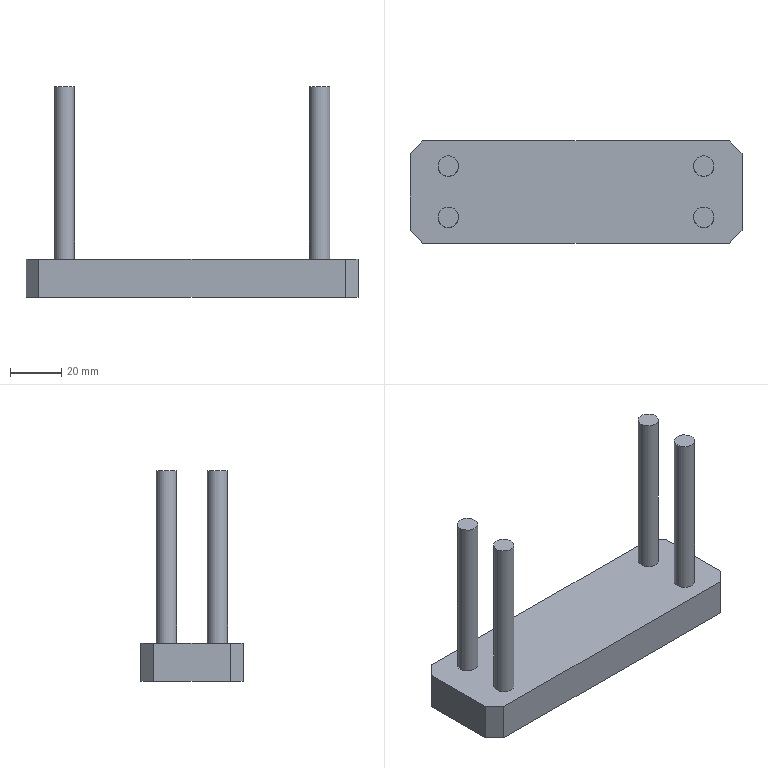Part | STEP file | Tube necking machine_id238_x_t | 1 solid | 18 faces | box 130 x 40 x 82.5 mm | volume 90822 mm3 | plane 14 | cylinder 4 | commonest cylinder face diameters 8 x4
STEP:
#1=CARTESIAN_POINT('',(0.,0.,0.));
#2=DIRECTION('',(0.,0.,1.));
#3=DIRECTION('',(1.,0.,0.));
#4=AXIS2_PLACEMENT_3D('',#1,#2,#3);
#5=CARTESIAN_POINT('',(-54.,60.,187.5));
#6=VERTEX_POINT('',#5);
#7=CARTESIAN_POINT('',(-46.,60.,187.5));
#8=VERTEX_POINT('',#7);
#9=CARTESIAN_POINT('',(-50.,60.,187.5));
#10=DIRECTION('',(0.,0.,-1.));
#11=DIRECTION('',(-1.,0.,0.));
#12=AXIS2_PLACEMENT_3D('',#9,#10,#11);
#13=CIRCLE('',#12,4.);
#14=CARTESIAN_POINT('',(-50.,60.,187.5));
#15=DIRECTION('',(0.,0.,-1.));
#16=DIRECTION('',(-1.,0.,0.));
#17=AXIS2_PLACEMENT_3D('',#14,#15,#16);
#18=PLANE('',#17);
#19=CARTESIAN_POINT('',(0.,0.));
#20=DIRECTION('',(1.,0.));
#21=AXIS2_PLACEMENT_2D('',#19,#20);
#22=CIRCLE('',#21,4.);
#23=(GEOMETRIC_REPRESENTATION_CONTEXT(2)PARAMETRIC_REPRESENTATION_CONTEXT()REPRESENTATION_CONTEXT('',''));
#24=DEFINITIONAL_REPRESENTATION('',(#22),#23);
#25=PCURVE('',#18,#24);
#26=CARTESIAN_POINT('',(-50.,60.,-489.65));
#27=DIRECTION('',(0.,0.,1.));
#28=DIRECTION('',(1.,0.,0.));
#29=AXIS2_PLACEMENT_3D('',#26,#27,#28);
#30=CYLINDRICAL_SURFACE('',#29,4.);
#31=CARTESIAN_POINT('',(3.142,677.15));
#32=DIRECTION('',(-1.,0.));
#33=VECTOR('',#32,1.);
#34=LINE('',#31,#33);
#35=(GEOMETRIC_REPRESENTATION_CONTEXT(2)PARAMETRIC_REPRESENTATION_CONTEXT()REPRESENTATION_CONTEXT('',''));
#36=DEFINITIONAL_REPRESENTATION('',(#34),#35);
#37=PCURVE('',#30,#36);
#38=SURFACE_CURVE('',#13,(#25,#37),.PCURVE_S1.);
#39=EDGE_CURVE('',#6,#8,#38,.T.);
#40=ORIENTED_EDGE('',*,*,#39,.F.);
#41=CARTESIAN_POINT('',(-50.,60.,187.5));
#42=DIRECTION('',(0.,0.,-1.));
#43=DIRECTION('',(-1.,0.,0.));
#44=AXIS2_PLACEMENT_3D('',#41,#42,#43);
#45=CIRCLE('',#44,4.);
#46=CARTESIAN_POINT('',(0.,0.));
#47=DIRECTION('',(1.,0.));
#48=AXIS2_PLACEMENT_2D('',#46,#47);
#49=CIRCLE('',#48,4.);
#50=(GEOMETRIC_REPRESENTATION_CONTEXT(2)PARAMETRIC_REPRESENTATION_CONTEXT()REPRESENTATION_CONTEXT('',''));
#51=DEFINITIONAL_REPRESENTATION('',(#49),#50);
#52=PCURVE('',#18,#51);
#53=CARTESIAN_POINT('',(9.425,677.15));
#54=DIRECTION('',(-1.,0.));
#55=VECTOR('',#54,1.);
#56=LINE('',#53,#55);
#57=(GEOMETRIC_REPRESENTATION_CONTEXT(2)PARAMETRIC_REPRESENTATION_CONTEXT()REPRESENTATION_CONTEXT('',''));
#58=DEFINITIONAL_REPRESENTATION('',(#56),#57);
#59=PCURVE('',#30,#58);
#60=SURFACE_CURVE('',#45,(#52,#59),.PCURVE_S1.);
#61=EDGE_CURVE('',#8,#6,#60,.T.);
#62=ORIENTED_EDGE('',*,*,#61,.F.);
#63=EDGE_LOOP('',(#40,#62));
#64=FACE_BOUND('',#63,.T.);
#65=ADVANCED_FACE('',(#64),#18,.F.);
#66=CARTESIAN_POINT('',(-46.,60.,120.));
#67=VERTEX_POINT('',#66);
#68=CARTESIAN_POINT('',(-50.,60.,120.));
#69=DIRECTION('',(0.,0.,1.));
#70=DIRECTION('',(1.,0.,0.));
#71=AXIS2_PLACEMENT_3D('',#68,#69,#70);
#72=CIRCLE('',#71,4.);
#73=CARTESIAN_POINT('',(0.,609.65));
#74=DIRECTION('',(1.,0.));
#75=VECTOR('',#74,1.);
#76=LINE('',#73,#75);
#77=(GEOMETRIC_REPRESENTATION_CONTEXT(2)PARAMETRIC_REPRESENTATION_CONTEXT()REPRESENTATION_CONTEXT('',''));
#78=DEFINITIONAL_REPRESENTATION('',(#76),#77);
#79=PCURVE('',#30,#78);
#80=CARTESIAN_POINT('',(0.,0.,120.));
#81=DIRECTION('',(0.,0.,1.));
#82=DIRECTION('',(1.,0.,0.));
#83=AXIS2_PLACEMENT_3D('',#80,#81,#82);
#84=PLANE('',#83);
#85=CARTESIAN_POINT('',(-50.,60.));
#86=DIRECTION('',(1.,0.));
#87=AXIS2_PLACEMENT_2D('',#85,#86);
#88=CIRCLE('',#87,4.);
#89=(GEOMETRIC_REPRESENTATION_CONTEXT(2)PARAMETRIC_REPRESENTATION_CONTEXT()REPRESENTATION_CONTEXT('',''));
#90=DEFINITIONAL_REPRESENTATION('',(#88),#89);
#91=PCURVE('',#84,#90);
#92=SURFACE_CURVE('',#72,(#79,#91),.PCURVE_S1.);
#93=EDGE_CURVE('',#67,#67,#92,.T.);
#94=ORIENTED_EDGE('',*,*,#93,.T.);
#95=CARTESIAN_POINT('',(-46.,60.,120.));
#96=CARTESIAN_POINT('',(-46.,60.,187.5));
#97=B_SPLINE_CURVE_WITH_KNOTS('',1,(#95,#96),.UNSPECIFIED.,.F.,.F.,(2,2),(609.65,677.15),.PIECEWISE_BEZIER_KNOTS.);
#98=CARTESIAN_POINT('',(6.283,0.));
#99=DIRECTION('',(0.,1.));
#100=VECTOR('',#99,1.);
#101=LINE('',#98,#100);
#102=(GEOMETRIC_REPRESENTATION_CONTEXT(2)PARAMETRIC_REPRESENTATION_CONTEXT()REPRESENTATION_CONTEXT('',''));
#103=DEFINITIONAL_REPRESENTATION('',(#101),#102);
#104=PCURVE('',#30,#103);
#105=CARTESIAN_POINT('',(0.,0.));
#106=DIRECTION('',(0.,1.));
#107=VECTOR('',#106,1.);
#108=LINE('',#105,#107);
#109=(GEOMETRIC_REPRESENTATION_CONTEXT(2)PARAMETRIC_REPRESENTATION_CONTEXT()REPRESENTATION_CONTEXT('',''));
#110=DEFINITIONAL_REPRESENTATION('',(#108),#109);
#111=PCURVE('',#30,#110);
#112=SEAM_CURVE('',#97,(#104,#111),.PCURVE_S1.);
#113=EDGE_CURVE('',#67,#8,#112,.T.);
#114=ORIENTED_EDGE('',*,*,#113,.T.);
#115=ORIENTED_EDGE('',*,*,#61,.T.);
#116=ORIENTED_EDGE('',*,*,#39,.T.);
#117=ORIENTED_EDGE('',*,*,#113,.F.);
#118=EDGE_LOOP('',(#94,#114,#115,#116,#117));
#119=FACE_BOUND('',#118,.T.);
#120=ADVANCED_FACE('',(#119),#30,.T.);
#121=CARTESIAN_POINT('',(-65.,65.,120.));
#122=VERTEX_POINT('',#121);
#123=CARTESIAN_POINT('',(-65.,35.,120.));
#124=VERTEX_POINT('',#123);
#125=CARTESIAN_POINT('',(-65.,70.,120.));
#126=DIRECTION('',(0.,-1.,0.));
#127=VECTOR('',#126,1.);
#128=LINE('',#125,#127);
#129=CARTESIAN_POINT('',(-65.,70.,120.));
#130=DIRECTION('',(1.,0.,0.));
#131=DIRECTION('',(0.,0.,-1.));
#132=AXIS2_PLACEMENT_3D('',#129,#130,#131);
#133=PLANE('',#132);
#134=CARTESIAN_POINT('',(0.,0.));
#135=DIRECTION('',(0.,-1.));
#136=VECTOR('',#135,1.);
#137=LINE('',#134,#136);
#138=(GEOMETRIC_REPRESENTATION_CONTEXT(2)PARAMETRIC_REPRESENTATION_CONTEXT()REPRESENTATION_CONTEXT('',''));
#139=DEFINITIONAL_REPRESENTATION('',(#137),#138);
#140=PCURVE('',#133,#139);
#141=CARTESIAN_POINT('',(-65.,70.));
#142=DIRECTION('',(0.,-1.));
#143=VECTOR('',#142,1.);
#144=LINE('',#141,#143);
#145=(GEOMETRIC_REPRESENTATION_CONTEXT(2)PARAMETRIC_REPRESENTATION_CONTEXT()REPRESENTATION_CONTEXT('',''));
#146=DEFINITIONAL_REPRESENTATION('',(#144),#145);
#147=PCURVE('',#84,#146);
#148=SURFACE_CURVE('',#128,(#140,#147),.PCURVE_S1.);
#149=EDGE_CURVE('',#122,#124,#148,.T.);
#150=ORIENTED_EDGE('',*,*,#149,.F.);
#151=CARTESIAN_POINT('',(-65.,65.,105.));
#152=VERTEX_POINT('',#151);
#153=CARTESIAN_POINT('',(-65.,65.,120.));
#154=DIRECTION('',(0.,0.,-1.));
#155=VECTOR('',#154,1.);
#156=LINE('',#153,#155);
#157=CARTESIAN_POINT('',(0.,-5.));
#158=DIRECTION('',(1.,0.));
#159=VECTOR('',#158,1.);
#160=LINE('',#157,#159);
#161=(GEOMETRIC_REPRESENTATION_CONTEXT(2)PARAMETRIC_REPRESENTATION_CONTEXT()REPRESENTATION_CONTEXT('',''));
#162=DEFINITIONAL_REPRESENTATION('',(#160),#161);
#163=PCURVE('',#133,#162);
#164=CARTESIAN_POINT('',(-65.,65.,120.));
#165=DIRECTION('',(0.7071,-0.7071,0.));
#166=DIRECTION('',(0.,0.,-1.));
#167=AXIS2_PLACEMENT_3D('',#164,#165,#166);
#168=PLANE('',#167);
#169=CARTESIAN_POINT('',(0.,0.));
#170=DIRECTION('',(1.,0.));
#171=VECTOR('',#170,1.);
#172=LINE('',#169,#171);
#173=(GEOMETRIC_REPRESENTATION_CONTEXT(2)PARAMETRIC_REPRESENTATION_CONTEXT()REPRESENTATION_CONTEXT('',''));
#174=DEFINITIONAL_REPRESENTATION('',(#172),#173);
#175=PCURVE('',#168,#174);
#176=SURFACE_CURVE('',#156,(#163,#175),.PCURVE_S1.);
#177=EDGE_CURVE('',#122,#152,#176,.T.);
#178=ORIENTED_EDGE('',*,*,#177,.T.);
#179=CARTESIAN_POINT('',(-65.,35.,105.));
#180=VERTEX_POINT('',#179);
#181=CARTESIAN_POINT('',(-65.,70.,105.));
#182=DIRECTION('',(0.,-1.,0.));
#183=VECTOR('',#182,1.);
#184=LINE('',#181,#183);
#185=CARTESIAN_POINT('',(15.,0.));
#186=DIRECTION('',(0.,-1.));
#187=VECTOR('',#186,1.);
#188=LINE('',#185,#187);
#189=(GEOMETRIC_REPRESENTATION_CONTEXT(2)PARAMETRIC_REPRESENTATION_CONTEXT()REPRESENTATION_CONTEXT('',''));
#190=DEFINITIONAL_REPRESENTATION('',(#188),#189);
#191=PCURVE('',#133,#190);
#192=CARTESIAN_POINT('',(0.,0.,105.));
#193=DIRECTION('',(0.,0.,1.));
#194=DIRECTION('',(1.,0.,0.));
#195=AXIS2_PLACEMENT_3D('',#192,#193,#194);
#196=PLANE('',#195);
#197=CARTESIAN_POINT('',(-65.,70.));
#198=DIRECTION('',(0.,-1.));
#199=VECTOR('',#198,1.);
#200=LINE('',#197,#199);
#201=(GEOMETRIC_REPRESENTATION_CONTEXT(2)PARAMETRIC_REPRESENTATION_CONTEXT()REPRESENTATION_CONTEXT('',''));
#202=DEFINITIONAL_REPRESENTATION('',(#200),#201);
#203=PCURVE('',#196,#202);
#204=SURFACE_CURVE('',#184,(#191,#203),.PCURVE_S1.);
#205=EDGE_CURVE('',#152,#180,#204,.T.);
#206=ORIENTED_EDGE('',*,*,#205,.T.);
#207=CARTESIAN_POINT('',(-65.,35.,120.));
#208=DIRECTION('',(0.,0.,1.));
#209=VECTOR('',#208,1.);
#210=LINE('',#207,#209);
#211=CARTESIAN_POINT('',(0.,-35.));
#212=DIRECTION('',(-1.,0.));
#213=VECTOR('',#212,1.);
#214=LINE('',#211,#213);
#215=(GEOMETRIC_REPRESENTATION_CONTEXT(2)PARAMETRIC_REPRESENTATION_CONTEXT()REPRESENTATION_CONTEXT('',''));
#216=DEFINITIONAL_REPRESENTATION('',(#214),#215);
#217=PCURVE('',#133,#216);
#218=CARTESIAN_POINT('',(-60.,30.,120.));
#219=DIRECTION('',(0.7071,0.7071,0.));
#220=DIRECTION('',(0.,0.,-1.));
#221=AXIS2_PLACEMENT_3D('',#218,#219,#220);
#222=PLANE('',#221);
#223=CARTESIAN_POINT('',(0.,7.071));
#224=DIRECTION('',(-1.,0.));
#225=VECTOR('',#224,1.);
#226=LINE('',#223,#225);
#227=(GEOMETRIC_REPRESENTATION_CONTEXT(2)PARAMETRIC_REPRESENTATION_CONTEXT()REPRESENTATION_CONTEXT('',''));
#228=DEFINITIONAL_REPRESENTATION('',(#226),#227);
#229=PCURVE('',#222,#228);
#230=SURFACE_CURVE('',#210,(#217,#229),.PCURVE_S1.);
#231=EDGE_CURVE('',#180,#124,#230,.T.);
#232=ORIENTED_EDGE('',*,*,#231,.T.);
#233=EDGE_LOOP('',(#150,#178,#206,#232));
#234=FACE_BOUND('',#233,.T.);
#235=ADVANCED_FACE('',(#234),#133,.F.);
#236=CARTESIAN_POINT('',(-60.,30.,120.));
#237=VERTEX_POINT('',#236);
#238=CARTESIAN_POINT('',(60.,30.,120.));
#239=VERTEX_POINT('',#238);
#240=CARTESIAN_POINT('',(-65.,30.,120.));
#241=DIRECTION('',(1.,0.,0.));
#242=VECTOR('',#241,1.);
#243=LINE('',#240,#242);
#244=CARTESIAN_POINT('',(-65.,30.,120.));
#245=DIRECTION('',(0.,1.,0.));
#246=DIRECTION('',(0.,0.,1.));
#247=AXIS2_PLACEMENT_3D('',#244,#245,#246);
#248=PLANE('',#247);
#249=CARTESIAN_POINT('',(0.,0.));
#250=DIRECTION('',(0.,1.));
#251=VECTOR('',#250,1.);
#252=LINE('',#249,#251);
#253=(GEOMETRIC_REPRESENTATION_CONTEXT(2)PARAMETRIC_REPRESENTATION_CONTEXT()REPRESENTATION_CONTEXT('',''));
#254=DEFINITIONAL_REPRESENTATION('',(#252),#253);
#255=PCURVE('',#248,#254);
#256=CARTESIAN_POINT('',(-65.,30.));
#257=DIRECTION('',(1.,0.));
#258=VECTOR('',#257,1.);
#259=LINE('',#256,#258);
#260=(GEOMETRIC_REPRESENTATION_CONTEXT(2)PARAMETRIC_REPRESENTATION_CONTEXT()REPRESENTATION_CONTEXT('',''));
#261=DEFINITIONAL_REPRESENTATION('',(#259),#260);
#262=PCURVE('',#84,#261);
#263=SURFACE_CURVE('',#243,(#255,#262),.PCURVE_S1.);
#264=EDGE_CURVE('',#237,#239,#263,.T.);
#265=ORIENTED_EDGE('',*,*,#264,.F.);
#266=CARTESIAN_POINT('',(-60.,30.,105.));
#267=VERTEX_POINT('',#266);
#268=CARTESIAN_POINT('',(-60.,30.,120.));
#269=DIRECTION('',(0.,0.,-1.));
#270=VECTOR('',#269,1.);
#271=LINE('',#268,#270);
#272=CARTESIAN_POINT('',(0.,5.));
#273=DIRECTION('',(-1.,0.));
#274=VECTOR('',#273,1.);
#275=LINE('',#272,#274);
#276=(GEOMETRIC_REPRESENTATION_CONTEXT(2)PARAMETRIC_REPRESENTATION_CONTEXT()REPRESENTATION_CONTEXT('',''));
#277=DEFINITIONAL_REPRESENTATION('',(#275),#276);
#278=PCURVE('',#248,#277);
#279=CARTESIAN_POINT('',(0.,0.));
#280=DIRECTION('',(1.,0.));
#281=VECTOR('',#280,1.);
#282=LINE('',#279,#281);
#283=(GEOMETRIC_REPRESENTATION_CONTEXT(2)PARAMETRIC_REPRESENTATION_CONTEXT()REPRESENTATION_CONTEXT('',''));
#284=DEFINITIONAL_REPRESENTATION('',(#282),#283);
#285=PCURVE('',#222,#284);
#286=SURFACE_CURVE('',#271,(#278,#285),.PCURVE_S1.);
#287=EDGE_CURVE('',#237,#267,#286,.T.);
#288=ORIENTED_EDGE('',*,*,#287,.T.);
#289=CARTESIAN_POINT('',(60.,30.,105.));
#290=VERTEX_POINT('',#289);
#291=CARTESIAN_POINT('',(-65.,30.,105.));
#292=DIRECTION('',(1.,0.,0.));
#293=VECTOR('',#292,1.);
#294=LINE('',#291,#293);
#295=CARTESIAN_POINT('',(-15.,0.));
#296=DIRECTION('',(0.,1.));
#297=VECTOR('',#296,1.);
#298=LINE('',#295,#297);
#299=(GEOMETRIC_REPRESENTATION_CONTEXT(2)PARAMETRIC_REPRESENTATION_CONTEXT()REPRESENTATION_CONTEXT('',''));
#300=DEFINITIONAL_REPRESENTATION('',(#298),#299);
#301=PCURVE('',#248,#300);
#302=CARTESIAN_POINT('',(-65.,30.));
#303=DIRECTION('',(1.,0.));
#304=VECTOR('',#303,1.);
#305=LINE('',#302,#304);
#306=(GEOMETRIC_REPRESENTATION_CONTEXT(2)PARAMETRIC_REPRESENTATION_CONTEXT()REPRESENTATION_CONTEXT('',''));
#307=DEFINITIONAL_REPRESENTATION('',(#305),#306);
#308=PCURVE('',#196,#307);
#309=SURFACE_CURVE('',#294,(#301,#308),.PCURVE_S1.);
#310=EDGE_CURVE('',#267,#290,#309,.T.);
#311=ORIENTED_EDGE('',*,*,#310,.T.);
#312=CARTESIAN_POINT('',(60.,30.,120.));
#313=DIRECTION('',(0.,0.,1.));
#314=VECTOR('',#313,1.);
#315=LINE('',#312,#314);
#316=CARTESIAN_POINT('',(0.,125.));
#317=DIRECTION('',(1.,0.));
#318=VECTOR('',#317,1.);
#319=LINE('',#316,#318);
#320=(GEOMETRIC_REPRESENTATION_CONTEXT(2)PARAMETRIC_REPRESENTATION_CONTEXT()REPRESENTATION_CONTEXT('',''));
#321=DEFINITIONAL_REPRESENTATION('',(#319),#320);
#322=PCURVE('',#248,#321);
#323=CARTESIAN_POINT('',(65.,35.,120.));
#324=DIRECTION('',(-0.7071,0.7071,0.));
#325=DIRECTION('',(0.,0.,-1.));
#326=AXIS2_PLACEMENT_3D('',#323,#324,#325);
#327=PLANE('',#326);
#328=CARTESIAN_POINT('',(0.,7.071));
#329=DIRECTION('',(-1.,0.));
#330=VECTOR('',#329,1.);
#331=LINE('',#328,#330);
#332=(GEOMETRIC_REPRESENTATION_CONTEXT(2)PARAMETRIC_REPRESENTATION_CONTEXT()REPRESENTATION_CONTEXT('',''));
#333=DEFINITIONAL_REPRESENTATION('',(#331),#332);
#334=PCURVE('',#327,#333);
#335=SURFACE_CURVE('',#315,(#322,#334),.PCURVE_S1.);
#336=EDGE_CURVE('',#290,#239,#335,.T.);
#337=ORIENTED_EDGE('',*,*,#336,.T.);
#338=EDGE_LOOP('',(#265,#288,#311,#337));
#339=FACE_BOUND('',#338,.T.);
#340=ADVANCED_FACE('',(#339),#248,.F.);
#341=CARTESIAN_POINT('',(65.,35.,105.));
#342=VERTEX_POINT('',#341);
#343=CARTESIAN_POINT('',(65.,65.,105.));
#344=VERTEX_POINT('',#343);
#345=CARTESIAN_POINT('',(65.,30.,105.));
#346=DIRECTION('',(0.,1.,0.));
#347=VECTOR('',#346,1.);
#348=LINE('',#345,#347);
#349=CARTESIAN_POINT('',(65.,30.,120.));
#350=DIRECTION('',(-1.,0.,0.));
#351=DIRECTION('',(0.,0.,1.));
#352=AXIS2_PLACEMENT_3D('',#349,#350,#351);
#353=PLANE('',#352);
#354=CARTESIAN_POINT('',(-15.,0.));
#355=DIRECTION('',(0.,1.));
#356=VECTOR('',#355,1.);
#357=LINE('',#354,#356);
#358=(GEOMETRIC_REPRESENTATION_CONTEXT(2)PARAMETRIC_REPRESENTATION_CONTEXT()REPRESENTATION_CONTEXT('',''));
#359=DEFINITIONAL_REPRESENTATION('',(#357),#358);
#360=PCURVE('',#353,#359);
#361=CARTESIAN_POINT('',(65.,30.));
#362=DIRECTION('',(0.,1.));
#363=VECTOR('',#362,1.);
#364=LINE('',#361,#363);
#365=(GEOMETRIC_REPRESENTATION_CONTEXT(2)PARAMETRIC_REPRESENTATION_CONTEXT()REPRESENTATION_CONTEXT('',''));
#366=DEFINITIONAL_REPRESENTATION('',(#364),#365);
#367=PCURVE('',#196,#366);
#368=SURFACE_CURVE('',#348,(#360,#367),.PCURVE_S1.);
#369=EDGE_CURVE('',#342,#344,#368,.T.);
#370=ORIENTED_EDGE('',*,*,#369,.T.);
#371=CARTESIAN_POINT('',(65.,65.,120.));
#372=VERTEX_POINT('',#371);
#373=CARTESIAN_POINT('',(65.,65.,120.));
#374=DIRECTION('',(0.,0.,1.));
#375=VECTOR('',#374,1.);
#376=LINE('',#373,#375);
#377=CARTESIAN_POINT('',(0.,35.));
#378=DIRECTION('',(1.,0.));
#379=VECTOR('',#378,1.);
#380=LINE('',#377,#379);
#381=(GEOMETRIC_REPRESENTATION_CONTEXT(2)PARAMETRIC_REPRESENTATION_CONTEXT()REPRESENTATION_CONTEXT('',''));
#382=DEFINITIONAL_REPRESENTATION('',(#380),#381);
#383=PCURVE('',#353,#382);
#384=CARTESIAN_POINT('',(60.,70.,120.));
#385=DIRECTION('',(-0.7071,-0.7071,0.));
#386=DIRECTION('',(0.,0.,-1.));
#387=AXIS2_PLACEMENT_3D('',#384,#385,#386);
#388=PLANE('',#387);
#389=CARTESIAN_POINT('',(0.,7.071));
#390=DIRECTION('',(-1.,0.));
#391=VECTOR('',#390,1.);
#392=LINE('',#389,#391);
#393=(GEOMETRIC_REPRESENTATION_CONTEXT(2)PARAMETRIC_REPRESENTATION_CONTEXT()REPRESENTATION_CONTEXT('',''));
#394=DEFINITIONAL_REPRESENTATION('',(#392),#393);
#395=PCURVE('',#388,#394);
#396=SURFACE_CURVE('',#376,(#383,#395),.PCURVE_S1.);
#397=EDGE_CURVE('',#344,#372,#396,.T.);
#398=ORIENTED_EDGE('',*,*,#397,.T.);
#399=CARTESIAN_POINT('',(65.,35.,120.));
#400=VERTEX_POINT('',#399);
#401=CARTESIAN_POINT('',(65.,30.,120.));
#402=DIRECTION('',(0.,1.,0.));
#403=VECTOR('',#402,1.);
#404=LINE('',#401,#403);
#405=CARTESIAN_POINT('',(0.,0.));
#406=DIRECTION('',(0.,1.));
#407=VECTOR('',#406,1.);
#408=LINE('',#405,#407);
#409=(GEOMETRIC_REPRESENTATION_CONTEXT(2)PARAMETRIC_REPRESENTATION_CONTEXT()REPRESENTATION_CONTEXT('',''));
#410=DEFINITIONAL_REPRESENTATION('',(#408),#409);
#411=PCURVE('',#353,#410);
#412=CARTESIAN_POINT('',(65.,30.));
#413=DIRECTION('',(0.,1.));
#414=VECTOR('',#413,1.);
#415=LINE('',#412,#414);
#416=(GEOMETRIC_REPRESENTATION_CONTEXT(2)PARAMETRIC_REPRESENTATION_CONTEXT()REPRESENTATION_CONTEXT('',''));
#417=DEFINITIONAL_REPRESENTATION('',(#415),#416);
#418=PCURVE('',#84,#417);
#419=SURFACE_CURVE('',#404,(#411,#418),.PCURVE_S1.);
#420=EDGE_CURVE('',#400,#372,#419,.T.);
#421=ORIENTED_EDGE('',*,*,#420,.F.);
#422=CARTESIAN_POINT('',(65.,35.,120.));
#423=DIRECTION('',(0.,0.,-1.));
#424=VECTOR('',#423,1.);
#425=LINE('',#422,#424);
#426=CARTESIAN_POINT('',(0.,5.));
#427=DIRECTION('',(-1.,0.));
#428=VECTOR('',#427,1.);
#429=LINE('',#426,#428);
#430=(GEOMETRIC_REPRESENTATION_CONTEXT(2)PARAMETRIC_REPRESENTATION_CONTEXT()REPRESENTATION_CONTEXT('',''));
#431=DEFINITIONAL_REPRESENTATION('',(#429),#430);
#432=PCURVE('',#353,#431);
#433=CARTESIAN_POINT('',(0.,0.));
#434=DIRECTION('',(1.,0.));
#435=VECTOR('',#434,1.);
#436=LINE('',#433,#435);
#437=(GEOMETRIC_REPRESENTATION_CONTEXT(2)PARAMETRIC_REPRESENTATION_CONTEXT()REPRESENTATION_CONTEXT('',''));
#438=DEFINITIONAL_REPRESENTATION('',(#436),#437);
#439=PCURVE('',#327,#438);
#440=SURFACE_CURVE('',#425,(#432,#439),.PCURVE_S1.);
#441=EDGE_CURVE('',#400,#342,#440,.T.);
#442=ORIENTED_EDGE('',*,*,#441,.T.);
#443=EDGE_LOOP('',(#370,#398,#421,#442));
#444=FACE_BOUND('',#443,.T.);
#445=ADVANCED_FACE('',(#444),#353,.F.);
#446=CARTESIAN_POINT('',(60.,70.,105.));
#447=VERTEX_POINT('',#446);
#448=CARTESIAN_POINT('',(-60.,70.,105.));
#449=VERTEX_POINT('',#448);
#450=CARTESIAN_POINT('',(65.,70.,105.));
#451=DIRECTION('',(-1.,0.,0.));
#452=VECTOR('',#451,1.);
#453=LINE('',#450,#452);
#454=CARTESIAN_POINT('',(65.,70.,120.));
#455=DIRECTION('',(0.,-1.,0.));
#456=DIRECTION('',(0.,0.,-1.));
#457=AXIS2_PLACEMENT_3D('',#454,#455,#456);
#458=PLANE('',#457);
#459=CARTESIAN_POINT('',(15.,0.));
#460=DIRECTION('',(0.,-1.));
#461=VECTOR('',#460,1.);
#462=LINE('',#459,#461);
#463=(GEOMETRIC_REPRESENTATION_CONTEXT(2)PARAMETRIC_REPRESENTATION_CONTEXT()REPRESENTATION_CONTEXT('',''));
#464=DEFINITIONAL_REPRESENTATION('',(#462),#463);
#465=PCURVE('',#458,#464);
#466=CARTESIAN_POINT('',(65.,70.));
#467=DIRECTION('',(-1.,0.));
#468=VECTOR('',#467,1.);
#469=LINE('',#466,#468);
#470=(GEOMETRIC_REPRESENTATION_CONTEXT(2)PARAMETRIC_REPRESENTATION_CONTEXT()REPRESENTATION_CONTEXT('',''));
#471=DEFINITIONAL_REPRESENTATION('',(#469),#470);
#472=PCURVE('',#196,#471);
#473=SURFACE_CURVE('',#453,(#465,#472),.PCURVE_S1.);
#474=EDGE_CURVE('',#447,#449,#473,.T.);
#475=ORIENTED_EDGE('',*,*,#474,.T.);
#476=CARTESIAN_POINT('',(-60.,70.,120.));
#477=VERTEX_POINT('',#476);
#478=CARTESIAN_POINT('',(-60.,70.,120.));
#479=DIRECTION('',(0.,0.,1.));
#480=VECTOR('',#479,1.);
#481=LINE('',#478,#480);
#482=CARTESIAN_POINT('',(0.,-125.));
#483=DIRECTION('',(-1.,0.));
#484=VECTOR('',#483,1.);
#485=LINE('',#482,#484);
#486=(GEOMETRIC_REPRESENTATION_CONTEXT(2)PARAMETRIC_REPRESENTATION_CONTEXT()REPRESENTATION_CONTEXT('',''));
#487=DEFINITIONAL_REPRESENTATION('',(#485),#486);
#488=PCURVE('',#458,#487);
#489=CARTESIAN_POINT('',(0.,7.071));
#490=DIRECTION('',(-1.,0.));
#491=VECTOR('',#490,1.);
#492=LINE('',#489,#491);
#493=(GEOMETRIC_REPRESENTATION_CONTEXT(2)PARAMETRIC_REPRESENTATION_CONTEXT()REPRESENTATION_CONTEXT('',''));
#494=DEFINITIONAL_REPRESENTATION('',(#492),#493);
#495=PCURVE('',#168,#494);
#496=SURFACE_CURVE('',#481,(#488,#495),.PCURVE_S1.);
#497=EDGE_CURVE('',#449,#477,#496,.T.);
#498=ORIENTED_EDGE('',*,*,#497,.T.);
#499=CARTESIAN_POINT('',(60.,70.,120.));
#500=VERTEX_POINT('',#499);
#501=CARTESIAN_POINT('',(65.,70.,120.));
#502=DIRECTION('',(-1.,0.,0.));
#503=VECTOR('',#502,1.);
#504=LINE('',#501,#503);
#505=CARTESIAN_POINT('',(0.,0.));
#506=DIRECTION('',(0.,-1.));
#507=VECTOR('',#506,1.);
#508=LINE('',#505,#507);
#509=(GEOMETRIC_REPRESENTATION_CONTEXT(2)PARAMETRIC_REPRESENTATION_CONTEXT()REPRESENTATION_CONTEXT('',''));
#510=DEFINITIONAL_REPRESENTATION('',(#508),#509);
#511=PCURVE('',#458,#510);
#512=CARTESIAN_POINT('',(65.,70.));
#513=DIRECTION('',(-1.,0.));
#514=VECTOR('',#513,1.);
#515=LINE('',#512,#514);
#516=(GEOMETRIC_REPRESENTATION_CONTEXT(2)PARAMETRIC_REPRESENTATION_CONTEXT()REPRESENTATION_CONTEXT('',''));
#517=DEFINITIONAL_REPRESENTATION('',(#515),#516);
#518=PCURVE('',#84,#517);
#519=SURFACE_CURVE('',#504,(#511,#518),.PCURVE_S1.);
#520=EDGE_CURVE('',#500,#477,#519,.T.);
#521=ORIENTED_EDGE('',*,*,#520,.F.);
#522=CARTESIAN_POINT('',(60.,70.,120.));
#523=DIRECTION('',(0.,0.,-1.));
#524=VECTOR('',#523,1.);
#525=LINE('',#522,#524);
#526=CARTESIAN_POINT('',(0.,-5.));
#527=DIRECTION('',(1.,0.));
#528=VECTOR('',#527,1.);
#529=LINE('',#526,#528);
#530=(GEOMETRIC_REPRESENTATION_CONTEXT(2)PARAMETRIC_REPRESENTATION_CONTEXT()REPRESENTATION_CONTEXT('',''));
#531=DEFINITIONAL_REPRESENTATION('',(#529),#530);
#532=PCURVE('',#458,#531);
#533=CARTESIAN_POINT('',(0.,0.));
#534=DIRECTION('',(1.,0.));
#535=VECTOR('',#534,1.);
#536=LINE('',#533,#535);
#537=(GEOMETRIC_REPRESENTATION_CONTEXT(2)PARAMETRIC_REPRESENTATION_CONTEXT()REPRESENTATION_CONTEXT('',''));
#538=DEFINITIONAL_REPRESENTATION('',(#536),#537);
#539=PCURVE('',#388,#538);
#540=SURFACE_CURVE('',#525,(#532,#539),.PCURVE_S1.);
#541=EDGE_CURVE('',#500,#447,#540,.T.);
#542=ORIENTED_EDGE('',*,*,#541,.T.);
#543=EDGE_LOOP('',(#475,#498,#521,#542));
#544=FACE_BOUND('',#543,.T.);
#545=ADVANCED_FACE('',(#544),#458,.F.);
#546=ORIENTED_EDGE('',*,*,#93,.F.);
#547=EDGE_LOOP('',(#546));
#548=FACE_BOUND('',#547,.T.);
#549=CARTESIAN_POINT('',(54.,60.,120.));
#550=VERTEX_POINT('',#549);
#551=CARTESIAN_POINT('',(50.,60.,120.));
#552=DIRECTION('',(0.,0.,1.));
#553=DIRECTION('',(1.,0.,0.));
#554=AXIS2_PLACEMENT_3D('',#551,#552,#553);
#555=CIRCLE('',#554,4.);
#556=CARTESIAN_POINT('',(50.,60.));
#557=DIRECTION('',(1.,0.));
#558=AXIS2_PLACEMENT_2D('',#556,#557);
#559=CIRCLE('',#558,4.);
#560=(GEOMETRIC_REPRESENTATION_CONTEXT(2)PARAMETRIC_REPRESENTATION_CONTEXT()REPRESENTATION_CONTEXT('',''));
#561=DEFINITIONAL_REPRESENTATION('',(#559),#560);
#562=PCURVE('',#84,#561);
#563=CARTESIAN_POINT('',(50.,60.,-489.65));
#564=DIRECTION('',(0.,0.,1.));
#565=DIRECTION('',(1.,0.,0.));
#566=AXIS2_PLACEMENT_3D('',#563,#564,#565);
#567=CYLINDRICAL_SURFACE('',#566,4.);
#568=CARTESIAN_POINT('',(0.,609.65));
#569=DIRECTION('',(1.,0.));
#570=VECTOR('',#569,1.);
#571=LINE('',#568,#570);
#572=(GEOMETRIC_REPRESENTATION_CONTEXT(2)PARAMETRIC_REPRESENTATION_CONTEXT()REPRESENTATION_CONTEXT('',''));
#573=DEFINITIONAL_REPRESENTATION('',(#571),#572);
#574=PCURVE('',#567,#573);
#575=SURFACE_CURVE('',#555,(#562,#574),.PCURVE_S1.);
#576=EDGE_CURVE('',#550,#550,#575,.T.);
#577=ORIENTED_EDGE('',*,*,#576,.F.);
#578=EDGE_LOOP('',(#577));
#579=FACE_BOUND('',#578,.T.);
#580=CARTESIAN_POINT('',(54.,40.,120.));
#581=VERTEX_POINT('',#580);
#582=CARTESIAN_POINT('',(50.,40.,120.));
#583=DIRECTION('',(0.,0.,-1.));
#584=DIRECTION('',(1.,0.,0.));
#585=AXIS2_PLACEMENT_3D('',#582,#583,#584);
#586=CIRCLE('',#585,4.);
#587=CARTESIAN_POINT('',(54.,40.));
#588=CARTESIAN_POINT('',(54.,33.072));
#589=CARTESIAN_POINT('',(48.,36.536));
#590=CARTESIAN_POINT('',(42.,40.));
#591=CARTESIAN_POINT('',(48.,43.464));
#592=CARTESIAN_POINT('',(54.,46.928));
#593=CARTESIAN_POINT('',(54.,40.));
#594=(BOUNDED_CURVE()B_SPLINE_CURVE(2,(#587,#588,#589,#590,#591,#592,#593),.UNSPECIFIED.,.T.,.F.)B_SPLINE_CURVE_WITH_KNOTS((1,2,2,2,2,1),(-2.094,0.,2.094,4.189,6.283,8.378),.UNSPECIFIED.)CURVE()GEOMETRIC_REPRESENTATION_ITEM()RATIONAL_B_SPLINE_CURVE((1.,0.5,1.,0.5,1.,0.5,1.))REPRESENTATION_ITEM(''));
#595=(GEOMETRIC_REPRESENTATION_CONTEXT(2)PARAMETRIC_REPRESENTATION_CONTEXT()REPRESENTATION_CONTEXT('',''));
#596=DEFINITIONAL_REPRESENTATION('',(#594),#595);
#597=PCURVE('',#84,#596);
#598=CARTESIAN_POINT('',(50.,40.,-489.65));
#599=DIRECTION('',(0.,0.,1.));
#600=DIRECTION('',(1.,0.,0.));
#601=AXIS2_PLACEMENT_3D('',#598,#599,#600);
#602=CYLINDRICAL_SURFACE('',#601,4.);
#603=CARTESIAN_POINT('',(6.283,609.65));
#604=DIRECTION('',(-1.,0.));
#605=VECTOR('',#604,1.);
#606=LINE('',#603,#605);
#607=(GEOMETRIC_REPRESENTATION_CONTEXT(2)PARAMETRIC_REPRESENTATION_CONTEXT()REPRESENTATION_CONTEXT('',''));
#608=DEFINITIONAL_REPRESENTATION('',(#606),#607);
#609=PCURVE('',#602,#608);
#610=SURFACE_CURVE('',#586,(#597,#609),.PCURVE_S1.);
#611=EDGE_CURVE('',#581,#581,#610,.T.);
#612=ORIENTED_EDGE('',*,*,#611,.T.);
#613=EDGE_LOOP('',(#612));
#614=FACE_BOUND('',#613,.T.);
#615=CARTESIAN_POINT('',(-46.,40.,120.));
#616=VERTEX_POINT('',#615);
#617=CARTESIAN_POINT('',(-50.,40.,120.));
#618=DIRECTION('',(0.,0.,1.));
#619=DIRECTION('',(1.,0.,0.));
#620=AXIS2_PLACEMENT_3D('',#617,#618,#619);
#621=CIRCLE('',#620,4.);
#622=CARTESIAN_POINT('',(-50.,40.));
#623=DIRECTION('',(1.,0.));
#624=AXIS2_PLACEMENT_2D('',#622,#623);
#625=CIRCLE('',#624,4.);
#626=(GEOMETRIC_REPRESENTATION_CONTEXT(2)PARAMETRIC_REPRESENTATION_CONTEXT()REPRESENTATION_CONTEXT('',''));
#627=DEFINITIONAL_REPRESENTATION('',(#625),#626);
#628=PCURVE('',#84,#627);
#629=CARTESIAN_POINT('',(-50.,40.,-489.65));
#630=DIRECTION('',(0.,0.,1.));
#631=DIRECTION('',(1.,0.,0.));
#632=AXIS2_PLACEMENT_3D('',#629,#630,#631);
#633=CYLINDRICAL_SURFACE('',#632,4.);
#634=CARTESIAN_POINT('',(0.,609.65));
#635=DIRECTION('',(1.,0.));
#636=VECTOR('',#635,1.);
#637=LINE('',#634,#636);
#638=(GEOMETRIC_REPRESENTATION_CONTEXT(2)PARAMETRIC_REPRESENTATION_CONTEXT()REPRESENTATION_CONTEXT('',''));
#639=DEFINITIONAL_REPRESENTATION('',(#637),#638);
#640=PCURVE('',#633,#639);
#641=SURFACE_CURVE('',#621,(#628,#640),.PCURVE_S1.);
#642=EDGE_CURVE('',#616,#616,#641,.T.);
#643=ORIENTED_EDGE('',*,*,#642,.F.);
#644=EDGE_LOOP('',(#643));
#645=FACE_BOUND('',#644,.T.);
#646=ORIENTED_EDGE('',*,*,#520,.T.);
#647=CARTESIAN_POINT('',(-65.,65.,120.));
#648=DIRECTION('',(-0.7071,-0.7071,0.));
#649=VECTOR('',#648,1.);
#650=LINE('',#647,#649);
#651=CARTESIAN_POINT('',(-65.,65.));
#652=DIRECTION('',(-0.7071,-0.7071));
#653=VECTOR('',#652,1.);
#654=LINE('',#651,#653);
#655=(GEOMETRIC_REPRESENTATION_CONTEXT(2)PARAMETRIC_REPRESENTATION_CONTEXT()REPRESENTATION_CONTEXT('',''));
#656=DEFINITIONAL_REPRESENTATION('',(#654),#655);
#657=PCURVE('',#84,#656);
#658=CARTESIAN_POINT('',(0.,0.));
#659=DIRECTION('',(0.,-1.));
#660=VECTOR('',#659,1.);
#661=LINE('',#658,#660);
#662=(GEOMETRIC_REPRESENTATION_CONTEXT(2)PARAMETRIC_REPRESENTATION_CONTEXT()REPRESENTATION_CONTEXT('',''));
#663=DEFINITIONAL_REPRESENTATION('',(#661),#662);
#664=PCURVE('',#168,#663);
#665=SURFACE_CURVE('',#650,(#657,#664),.PCURVE_S1.);
#666=EDGE_CURVE('',#477,#122,#665,.T.);
#667=ORIENTED_EDGE('',*,*,#666,.T.);
#668=ORIENTED_EDGE('',*,*,#149,.T.);
#669=CARTESIAN_POINT('',(-15.,-15.,120.));
#670=DIRECTION('',(0.7071,-0.7071,0.));
#671=VECTOR('',#670,1.);
#672=LINE('',#669,#671);
#673=CARTESIAN_POINT('',(-15.,-15.));
#674=DIRECTION('',(0.7071,-0.7071));
#675=VECTOR('',#674,1.);
#676=LINE('',#673,#675);
#677=(GEOMETRIC_REPRESENTATION_CONTEXT(2)PARAMETRIC_REPRESENTATION_CONTEXT()REPRESENTATION_CONTEXT('',''));
#678=DEFINITIONAL_REPRESENTATION('',(#676),#677);
#679=PCURVE('',#84,#678);
#680=CARTESIAN_POINT('',(0.,-63.64));
#681=DIRECTION('',(0.,-1.));
#682=VECTOR('',#681,1.);
#683=LINE('',#680,#682);
#684=(GEOMETRIC_REPRESENTATION_CONTEXT(2)PARAMETRIC_REPRESENTATION_CONTEXT()REPRESENTATION_CONTEXT('',''));
#685=DEFINITIONAL_REPRESENTATION('',(#683),#684);
#686=PCURVE('',#222,#685);
#687=SURFACE_CURVE('',#672,(#679,#686),.PCURVE_S1.);
#688=EDGE_CURVE('',#124,#237,#687,.T.);
#689=ORIENTED_EDGE('',*,*,#688,.T.);
#690=ORIENTED_EDGE('',*,*,#264,.T.);
#691=CARTESIAN_POINT('',(15.,-15.,120.));
#692=DIRECTION('',(0.7071,0.7071,0.));
#693=VECTOR('',#692,1.);
#694=LINE('',#691,#693);
#695=CARTESIAN_POINT('',(15.,-15.));
#696=DIRECTION('',(0.7071,0.7071));
#697=VECTOR('',#696,1.);
#698=LINE('',#695,#697);
#699=(GEOMETRIC_REPRESENTATION_CONTEXT(2)PARAMETRIC_REPRESENTATION_CONTEXT()REPRESENTATION_CONTEXT('',''));
#700=DEFINITIONAL_REPRESENTATION('',(#698),#699);
#701=PCURVE('',#84,#700);
#702=CARTESIAN_POINT('',(0.,70.711));
#703=DIRECTION('',(0.,-1.));
#704=VECTOR('',#703,1.);
#705=LINE('',#702,#704);
#706=(GEOMETRIC_REPRESENTATION_CONTEXT(2)PARAMETRIC_REPRESENTATION_CONTEXT()REPRESENTATION_CONTEXT('',''));
#707=DEFINITIONAL_REPRESENTATION('',(#705),#706);
#708=PCURVE('',#327,#707);
#709=SURFACE_CURVE('',#694,(#701,#708),.PCURVE_S1.);
#710=EDGE_CURVE('',#239,#400,#709,.T.);
#711=ORIENTED_EDGE('',*,*,#710,.T.);
#712=ORIENTED_EDGE('',*,*,#420,.T.);
#713=CARTESIAN_POINT('',(65.,65.,120.));
#714=DIRECTION('',(-0.7071,0.7071,0.));
#715=VECTOR('',#714,1.);
#716=LINE('',#713,#715);
#717=CARTESIAN_POINT('',(65.,65.));
#718=DIRECTION('',(-0.7071,0.7071));
#719=VECTOR('',#718,1.);
#720=LINE('',#717,#719);
#721=(GEOMETRIC_REPRESENTATION_CONTEXT(2)PARAMETRIC_REPRESENTATION_CONTEXT()REPRESENTATION_CONTEXT('',''));
#722=DEFINITIONAL_REPRESENTATION('',(#720),#721);
#723=PCURVE('',#84,#722);
#724=CARTESIAN_POINT('',(0.,7.071));
#725=DIRECTION('',(0.,-1.));
#726=VECTOR('',#725,1.);
#727=LINE('',#724,#726);
#728=(GEOMETRIC_REPRESENTATION_CONTEXT(2)PARAMETRIC_REPRESENTATION_CONTEXT()REPRESENTATION_CONTEXT('',''));
#729=DEFINITIONAL_REPRESENTATION('',(#727),#728);
#730=PCURVE('',#388,#729);
#731=SURFACE_CURVE('',#716,(#723,#730),.PCURVE_S1.);
#732=EDGE_CURVE('',#372,#500,#731,.T.);
#733=ORIENTED_EDGE('',*,*,#732,.T.);
#734=EDGE_LOOP('',(#646,#667,#668,#689,#690,#711,#712,#733));
#735=FACE_BOUND('',#734,.T.);
#736=ADVANCED_FACE('',(#548,#579,#614,#645,#735),#84,.T.);
#737=ORIENTED_EDGE('',*,*,#205,.F.);
#738=CARTESIAN_POINT('',(-65.,65.,105.));
#739=DIRECTION('',(0.7071,0.7071,0.));
#740=VECTOR('',#739,1.);
#741=LINE('',#738,#740);
#742=CARTESIAN_POINT('',(-65.,65.));
#743=DIRECTION('',(0.7071,0.7071));
#744=VECTOR('',#743,1.);
#745=LINE('',#742,#744);
#746=(GEOMETRIC_REPRESENTATION_CONTEXT(2)PARAMETRIC_REPRESENTATION_CONTEXT()REPRESENTATION_CONTEXT('',''));
#747=DEFINITIONAL_REPRESENTATION('',(#745),#746);
#748=PCURVE('',#196,#747);
#749=CARTESIAN_POINT('',(15.,0.));
#750=DIRECTION('',(0.,1.));
#751=VECTOR('',#750,1.);
#752=LINE('',#749,#751);
#753=(GEOMETRIC_REPRESENTATION_CONTEXT(2)PARAMETRIC_REPRESENTATION_CONTEXT()REPRESENTATION_CONTEXT('',''));
#754=DEFINITIONAL_REPRESENTATION('',(#752),#753);
#755=PCURVE('',#168,#754);
#756=SURFACE_CURVE('',#741,(#748,#755),.PCURVE_S1.);
#757=EDGE_CURVE('',#152,#449,#756,.T.);
#758=ORIENTED_EDGE('',*,*,#757,.T.);
#759=ORIENTED_EDGE('',*,*,#474,.F.);
#760=CARTESIAN_POINT('',(60.,70.,105.));
#761=DIRECTION('',(0.7071,-0.7071,0.));
#762=VECTOR('',#761,1.);
#763=LINE('',#760,#762);
#764=CARTESIAN_POINT('',(60.,70.));
#765=DIRECTION('',(0.7071,-0.7071));
#766=VECTOR('',#765,1.);
#767=LINE('',#764,#766);
#768=(GEOMETRIC_REPRESENTATION_CONTEXT(2)PARAMETRIC_REPRESENTATION_CONTEXT()REPRESENTATION_CONTEXT('',''));
#769=DEFINITIONAL_REPRESENTATION('',(#767),#768);
#770=PCURVE('',#196,#769);
#771=CARTESIAN_POINT('',(15.,0.));
#772=DIRECTION('',(0.,1.));
#773=VECTOR('',#772,1.);
#774=LINE('',#771,#773);
#775=(GEOMETRIC_REPRESENTATION_CONTEXT(2)PARAMETRIC_REPRESENTATION_CONTEXT()REPRESENTATION_CONTEXT('',''));
#776=DEFINITIONAL_REPRESENTATION('',(#774),#775);
#777=PCURVE('',#388,#776);
#778=SURFACE_CURVE('',#763,(#770,#777),.PCURVE_S1.);
#779=EDGE_CURVE('',#447,#344,#778,.T.);
#780=ORIENTED_EDGE('',*,*,#779,.T.);
#781=ORIENTED_EDGE('',*,*,#369,.F.);
#782=CARTESIAN_POINT('',(65.,35.,105.));
#783=DIRECTION('',(-0.7071,-0.7071,0.));
#784=VECTOR('',#783,1.);
#785=LINE('',#782,#784);
#786=CARTESIAN_POINT('',(65.,35.));
#787=DIRECTION('',(-0.7071,-0.7071));
#788=VECTOR('',#787,1.);
#789=LINE('',#786,#788);
#790=(GEOMETRIC_REPRESENTATION_CONTEXT(2)PARAMETRIC_REPRESENTATION_CONTEXT()REPRESENTATION_CONTEXT('',''));
#791=DEFINITIONAL_REPRESENTATION('',(#789),#790);
#792=PCURVE('',#196,#791);
#793=CARTESIAN_POINT('',(15.,0.));
#794=DIRECTION('',(0.,1.));
#795=VECTOR('',#794,1.);
#796=LINE('',#793,#795);
#797=(GEOMETRIC_REPRESENTATION_CONTEXT(2)PARAMETRIC_REPRESENTATION_CONTEXT()REPRESENTATION_CONTEXT('',''));
#798=DEFINITIONAL_REPRESENTATION('',(#796),#797);
#799=PCURVE('',#327,#798);
#800=SURFACE_CURVE('',#785,(#792,#799),.PCURVE_S1.);
#801=EDGE_CURVE('',#342,#290,#800,.T.);
#802=ORIENTED_EDGE('',*,*,#801,.T.);
#803=ORIENTED_EDGE('',*,*,#310,.F.);
#804=CARTESIAN_POINT('',(-60.,30.,105.));
#805=DIRECTION('',(-0.7071,0.7071,0.));
#806=VECTOR('',#805,1.);
#807=LINE('',#804,#806);
#808=CARTESIAN_POINT('',(-60.,30.));
#809=DIRECTION('',(-0.7071,0.7071));
#810=VECTOR('',#809,1.);
#811=LINE('',#808,#810);
#812=(GEOMETRIC_REPRESENTATION_CONTEXT(2)PARAMETRIC_REPRESENTATION_CONTEXT()REPRESENTATION_CONTEXT('',''));
#813=DEFINITIONAL_REPRESENTATION('',(#811),#812);
#814=PCURVE('',#196,#813);
#815=CARTESIAN_POINT('',(15.,0.));
#816=DIRECTION('',(0.,1.));
#817=VECTOR('',#816,1.);
#818=LINE('',#815,#817);
#819=(GEOMETRIC_REPRESENTATION_CONTEXT(2)PARAMETRIC_REPRESENTATION_CONTEXT()REPRESENTATION_CONTEXT('',''));
#820=DEFINITIONAL_REPRESENTATION('',(#818),#819);
#821=PCURVE('',#222,#820);
#822=SURFACE_CURVE('',#807,(#814,#821),.PCURVE_S1.);
#823=EDGE_CURVE('',#267,#180,#822,.T.);
#824=ORIENTED_EDGE('',*,*,#823,.T.);
#825=EDGE_LOOP('',(#737,#758,#759,#780,#781,#802,#803,#824));
#826=FACE_BOUND('',#825,.T.);
#827=ADVANCED_FACE('',(#826),#196,.F.);
#828=ORIENTED_EDGE('',*,*,#666,.F.);
#829=ORIENTED_EDGE('',*,*,#497,.F.);
#830=ORIENTED_EDGE('',*,*,#757,.F.);
#831=ORIENTED_EDGE('',*,*,#177,.F.);
#832=EDGE_LOOP('',(#828,#829,#830,#831));
#833=FACE_BOUND('',#832,.T.);
#834=ADVANCED_FACE('',(#833),#168,.F.);
#835=ORIENTED_EDGE('',*,*,#688,.F.);
#836=ORIENTED_EDGE('',*,*,#231,.F.);
#837=ORIENTED_EDGE('',*,*,#823,.F.);
#838=ORIENTED_EDGE('',*,*,#287,.F.);
#839=EDGE_LOOP('',(#835,#836,#837,#838));
#840=FACE_BOUND('',#839,.T.);
#841=ADVANCED_FACE('',(#840),#222,.F.);
#842=ORIENTED_EDGE('',*,*,#732,.F.);
#843=ORIENTED_EDGE('',*,*,#397,.F.);
#844=ORIENTED_EDGE('',*,*,#779,.F.);
#845=ORIENTED_EDGE('',*,*,#541,.F.);
#846=EDGE_LOOP('',(#842,#843,#844,#845));
#847=FACE_BOUND('',#846,.T.);
#848=ADVANCED_FACE('',(#847),#388,.F.);
#849=ORIENTED_EDGE('',*,*,#710,.F.);
#850=ORIENTED_EDGE('',*,*,#336,.F.);
#851=ORIENTED_EDGE('',*,*,#801,.F.);
#852=ORIENTED_EDGE('',*,*,#441,.F.);
#853=EDGE_LOOP('',(#849,#850,#851,#852));
#854=FACE_BOUND('',#853,.T.);
#855=ADVANCED_FACE('',(#854),#327,.F.);
#856=CARTESIAN_POINT('',(-54.,40.,187.5));
#857=VERTEX_POINT('',#856);
#858=CARTESIAN_POINT('',(-46.,40.,187.5));
#859=VERTEX_POINT('',#858);
#860=CARTESIAN_POINT('',(-50.,40.,187.5));
#861=DIRECTION('',(0.,0.,-1.));
#862=DIRECTION('',(-1.,0.,0.));
#863=AXIS2_PLACEMENT_3D('',#860,#861,#862);
#864=CIRCLE('',#863,4.);
#865=CARTESIAN_POINT('',(-50.,40.,187.5));
#866=DIRECTION('',(0.,0.,-1.));
#867=DIRECTION('',(-1.,0.,0.));
#868=AXIS2_PLACEMENT_3D('',#865,#866,#867);
#869=PLANE('',#868);
#870=CARTESIAN_POINT('',(0.,0.));
#871=DIRECTION('',(1.,0.));
#872=AXIS2_PLACEMENT_2D('',#870,#871);
#873=CIRCLE('',#872,4.);
#874=(GEOMETRIC_REPRESENTATION_CONTEXT(2)PARAMETRIC_REPRESENTATION_CONTEXT()REPRESENTATION_CONTEXT('',''));
#875=DEFINITIONAL_REPRESENTATION('',(#873),#874);
#876=PCURVE('',#869,#875);
#877=CARTESIAN_POINT('',(3.142,677.15));
#878=DIRECTION('',(-1.,0.));
#879=VECTOR('',#878,1.);
#880=LINE('',#877,#879);
#881=(GEOMETRIC_REPRESENTATION_CONTEXT(2)PARAMETRIC_REPRESENTATION_CONTEXT()REPRESENTATION_CONTEXT('',''));
#882=DEFINITIONAL_REPRESENTATION('',(#880),#881);
#883=PCURVE('',#633,#882);
#884=SURFACE_CURVE('',#864,(#876,#883),.PCURVE_S1.);
#885=EDGE_CURVE('',#857,#859,#884,.T.);
#886=ORIENTED_EDGE('',*,*,#885,.F.);
#887=CARTESIAN_POINT('',(-50.,40.,187.5));
#888=DIRECTION('',(0.,0.,-1.));
#889=DIRECTION('',(-1.,0.,0.));
#890=AXIS2_PLACEMENT_3D('',#887,#888,#889);
#891=CIRCLE('',#890,4.);
#892=CARTESIAN_POINT('',(0.,0.));
#893=DIRECTION('',(1.,0.));
#894=AXIS2_PLACEMENT_2D('',#892,#893);
#895=CIRCLE('',#894,4.);
#896=(GEOMETRIC_REPRESENTATION_CONTEXT(2)PARAMETRIC_REPRESENTATION_CONTEXT()REPRESENTATION_CONTEXT('',''));
#897=DEFINITIONAL_REPRESENTATION('',(#895),#896);
#898=PCURVE('',#869,#897);
#899=CARTESIAN_POINT('',(9.425,677.15));
#900=DIRECTION('',(-1.,0.));
#901=VECTOR('',#900,1.);
#902=LINE('',#899,#901);
#903=(GEOMETRIC_REPRESENTATION_CONTEXT(2)PARAMETRIC_REPRESENTATION_CONTEXT()REPRESENTATION_CONTEXT('',''));
#904=DEFINITIONAL_REPRESENTATION('',(#902),#903);
#905=PCURVE('',#633,#904);
#906=SURFACE_CURVE('',#891,(#898,#905),.PCURVE_S1.);
#907=EDGE_CURVE('',#859,#857,#906,.T.);
#908=ORIENTED_EDGE('',*,*,#907,.F.);
#909=EDGE_LOOP('',(#886,#908));
#910=FACE_BOUND('',#909,.T.);
#911=ADVANCED_FACE('',(#910),#869,.F.);
#912=ORIENTED_EDGE('',*,*,#642,.T.);
#913=CARTESIAN_POINT('',(-46.,40.,120.));
#914=CARTESIAN_POINT('',(-46.,40.,187.5));
#915=B_SPLINE_CURVE_WITH_KNOTS('',1,(#913,#914),.UNSPECIFIED.,.F.,.F.,(2,2),(609.65,677.15),.PIECEWISE_BEZIER_KNOTS.);
#916=CARTESIAN_POINT('',(6.283,0.));
#917=DIRECTION('',(0.,1.));
#918=VECTOR('',#917,1.);
#919=LINE('',#916,#918);
#920=(GEOMETRIC_REPRESENTATION_CONTEXT(2)PARAMETRIC_REPRESENTATION_CONTEXT()REPRESENTATION_CONTEXT('',''));
#921=DEFINITIONAL_REPRESENTATION('',(#919),#920);
#922=PCURVE('',#633,#921);
#923=CARTESIAN_POINT('',(0.,0.));
#924=DIRECTION('',(0.,1.));
#925=VECTOR('',#924,1.);
#926=LINE('',#923,#925);
#927=(GEOMETRIC_REPRESENTATION_CONTEXT(2)PARAMETRIC_REPRESENTATION_CONTEXT()REPRESENTATION_CONTEXT('',''));
#928=DEFINITIONAL_REPRESENTATION('',(#926),#927);
#929=PCURVE('',#633,#928);
#930=SEAM_CURVE('',#915,(#922,#929),.PCURVE_S1.);
#931=EDGE_CURVE('',#616,#859,#930,.T.);
#932=ORIENTED_EDGE('',*,*,#931,.T.);
#933=ORIENTED_EDGE('',*,*,#907,.T.);
#934=ORIENTED_EDGE('',*,*,#885,.T.);
#935=ORIENTED_EDGE('',*,*,#931,.F.);
#936=EDGE_LOOP('',(#912,#932,#933,#934,#935));
#937=FACE_BOUND('',#936,.T.);
#938=ADVANCED_FACE('',(#937),#633,.T.);
#939=ORIENTED_EDGE('',*,*,#611,.F.);
#940=CARTESIAN_POINT('',(54.,40.,187.5));
#941=VERTEX_POINT('',#940);
#942=CARTESIAN_POINT('',(54.,40.,120.));
#943=CARTESIAN_POINT('',(54.,40.,187.5));
#944=B_SPLINE_CURVE_WITH_KNOTS('',1,(#942,#943),.UNSPECIFIED.,.F.,.F.,(2,2),(609.65,677.15),.PIECEWISE_BEZIER_KNOTS.);
#945=CARTESIAN_POINT('',(6.283,0.));
#946=DIRECTION('',(0.,1.));
#947=VECTOR('',#946,1.);
#948=LINE('',#945,#947);
#949=(GEOMETRIC_REPRESENTATION_CONTEXT(2)PARAMETRIC_REPRESENTATION_CONTEXT()REPRESENTATION_CONTEXT('',''));
#950=DEFINITIONAL_REPRESENTATION('',(#948),#949);
#951=PCURVE('',#602,#950);
#952=CARTESIAN_POINT('',(0.,0.));
#953=DIRECTION('',(0.,1.));
#954=VECTOR('',#953,1.);
#955=LINE('',#952,#954);
#956=(GEOMETRIC_REPRESENTATION_CONTEXT(2)PARAMETRIC_REPRESENTATION_CONTEXT()REPRESENTATION_CONTEXT('',''));
#957=DEFINITIONAL_REPRESENTATION('',(#955),#956);
#958=PCURVE('',#602,#957);
#959=SEAM_CURVE('',#944,(#951,#958),.PCURVE_S1.);
#960=EDGE_CURVE('',#581,#941,#959,.T.);
#961=ORIENTED_EDGE('',*,*,#960,.T.);
#962=CARTESIAN_POINT('',(50.,40.,187.5));
#963=DIRECTION('',(0.,0.,1.));
#964=DIRECTION('',(1.,0.,0.));
#965=AXIS2_PLACEMENT_3D('',#962,#963,#964);
#966=CIRCLE('',#965,4.);
#967=CARTESIAN_POINT('',(0.,677.15));
#968=DIRECTION('',(1.,0.));
#969=VECTOR('',#968,1.);
#970=LINE('',#967,#969);
#971=(GEOMETRIC_REPRESENTATION_CONTEXT(2)PARAMETRIC_REPRESENTATION_CONTEXT()REPRESENTATION_CONTEXT('',''));
#972=DEFINITIONAL_REPRESENTATION('',(#970),#971);
#973=PCURVE('',#602,#972);
#974=CARTESIAN_POINT('',(50.,40.,187.5));
#975=DIRECTION('',(0.,0.,1.));
#976=DIRECTION('',(1.,0.,0.));
#977=AXIS2_PLACEMENT_3D('',#974,#975,#976);
#978=PLANE('',#977);
#979=CARTESIAN_POINT('',(0.,0.));
#980=DIRECTION('',(1.,0.));
#981=AXIS2_PLACEMENT_2D('',#979,#980);
#982=CIRCLE('',#981,4.);
#983=(GEOMETRIC_REPRESENTATION_CONTEXT(2)PARAMETRIC_REPRESENTATION_CONTEXT()REPRESENTATION_CONTEXT('',''));
#984=DEFINITIONAL_REPRESENTATION('',(#982),#983);
#985=PCURVE('',#978,#984);
#986=SURFACE_CURVE('',#966,(#973,#985),.PCURVE_S1.);
#987=EDGE_CURVE('',#941,#941,#986,.T.);
#988=ORIENTED_EDGE('',*,*,#987,.F.);
#989=ORIENTED_EDGE('',*,*,#960,.F.);
#990=EDGE_LOOP('',(#939,#961,#988,#989));
#991=FACE_BOUND('',#990,.T.);
#992=ADVANCED_FACE('',(#991),#602,.T.);
#993=ORIENTED_EDGE('',*,*,#987,.T.);
#994=EDGE_LOOP('',(#993));
#995=FACE_BOUND('',#994,.T.);
#996=ADVANCED_FACE('',(#995),#978,.T.);
#997=CARTESIAN_POINT('',(46.,60.,187.5));
#998=VERTEX_POINT('',#997);
#999=CARTESIAN_POINT('',(54.,60.,187.5));
#1000=VERTEX_POINT('',#999);
#1001=CARTESIAN_POINT('',(50.,60.,187.5));
#1002=DIRECTION('',(0.,0.,-1.));
#1003=DIRECTION('',(-1.,0.,0.));
#1004=AXIS2_PLACEMENT_3D('',#1001,#1002,#1003);
#1005=CIRCLE('',#1004,4.);
#1006=CARTESIAN_POINT('',(50.,60.,187.5));
#1007=DIRECTION('',(0.,0.,-1.));
#1008=DIRECTION('',(-1.,0.,0.));
#1009=AXIS2_PLACEMENT_3D('',#1006,#1007,#1008);
#1010=PLANE('',#1009);
#1011=CARTESIAN_POINT('',(0.,0.));
#1012=DIRECTION('',(1.,0.));
#1013=AXIS2_PLACEMENT_2D('',#1011,#1012);
#1014=CIRCLE('',#1013,4.);
#1015=(GEOMETRIC_REPRESENTATION_CONTEXT(2)PARAMETRIC_REPRESENTATION_CONTEXT()REPRESENTATION_CONTEXT('',''));
#1016=DEFINITIONAL_REPRESENTATION('',(#1014),#1015);
#1017=PCURVE('',#1010,#1016);
#1018=CARTESIAN_POINT('',(3.142,677.15));
#1019=DIRECTION('',(-1.,0.));
#1020=VECTOR('',#1019,1.);
#1021=LINE('',#1018,#1020);
#1022=(GEOMETRIC_REPRESENTATION_CONTEXT(2)PARAMETRIC_REPRESENTATION_CONTEXT()REPRESENTATION_CONTEXT('',''));
#1023=DEFINITIONAL_REPRESENTATION('',(#1021),#1022);
#1024=PCURVE('',#567,#1023);
#1025=SURFACE_CURVE('',#1005,(#1017,#1024),.PCURVE_S1.);
#1026=EDGE_CURVE('',#998,#1000,#1025,.T.);
#1027=ORIENTED_EDGE('',*,*,#1026,.F.);
#1028=CARTESIAN_POINT('',(50.,60.,187.5));
#1029=DIRECTION('',(0.,0.,-1.));
#1030=DIRECTION('',(-1.,0.,0.));
#1031=AXIS2_PLACEMENT_3D('',#1028,#1029,#1030);
#1032=CIRCLE('',#1031,4.);
#1033=CARTESIAN_POINT('',(0.,0.));
#1034=DIRECTION('',(1.,0.));
#1035=AXIS2_PLACEMENT_2D('',#1033,#1034);
#1036=CIRCLE('',#1035,4.);
#1037=(GEOMETRIC_REPRESENTATION_CONTEXT(2)PARAMETRIC_REPRESENTATION_CONTEXT()REPRESENTATION_CONTEXT('',''));
#1038=DEFINITIONAL_REPRESENTATION('',(#1036),#1037);
#1039=PCURVE('',#1010,#1038);
#1040=CARTESIAN_POINT('',(9.425,677.15));
#1041=DIRECTION('',(-1.,0.));
#1042=VECTOR('',#1041,1.);
#1043=LINE('',#1040,#1042);
#1044=(GEOMETRIC_REPRESENTATION_CONTEXT(2)PARAMETRIC_REPRESENTATION_CONTEXT()REPRESENTATION_CONTEXT('',''));
#1045=DEFINITIONAL_REPRESENTATION('',(#1043),#1044);
#1046=PCURVE('',#567,#1045);
#1047=SURFACE_CURVE('',#1032,(#1039,#1046),.PCURVE_S1.);
#1048=EDGE_CURVE('',#1000,#998,#1047,.T.);
#1049=ORIENTED_EDGE('',*,*,#1048,.F.);
#1050=EDGE_LOOP('',(#1027,#1049));
#1051=FACE_BOUND('',#1050,.T.);
#1052=ADVANCED_FACE('',(#1051),#1010,.F.);
#1053=ORIENTED_EDGE('',*,*,#576,.T.);
#1054=CARTESIAN_POINT('',(54.,60.,120.));
#1055=CARTESIAN_POINT('',(54.,60.,187.5));
#1056=B_SPLINE_CURVE_WITH_KNOTS('',1,(#1054,#1055),.UNSPECIFIED.,.F.,.F.,(2,2),(609.65,677.15),.PIECEWISE_BEZIER_KNOTS.);
#1057=CARTESIAN_POINT('',(6.283,0.));
#1058=DIRECTION('',(0.,1.));
#1059=VECTOR('',#1058,1.);
#1060=LINE('',#1057,#1059);
#1061=(GEOMETRIC_REPRESENTATION_CONTEXT(2)PARAMETRIC_REPRESENTATION_CONTEXT()REPRESENTATION_CONTEXT('',''));
#1062=DEFINITIONAL_REPRESENTATION('',(#1060),#1061);
#1063=PCURVE('',#567,#1062);
#1064=CARTESIAN_POINT('',(0.,0.));
#1065=DIRECTION('',(0.,1.));
#1066=VECTOR('',#1065,1.);
#1067=LINE('',#1064,#1066);
#1068=(GEOMETRIC_REPRESENTATION_CONTEXT(2)PARAMETRIC_REPRESENTATION_CONTEXT()REPRESENTATION_CONTEXT('',''));
#1069=DEFINITIONAL_REPRESENTATION('',(#1067),#1068);
#1070=PCURVE('',#567,#1069);
#1071=SEAM_CURVE('',#1056,(#1063,#1070),.PCURVE_S1.);
#1072=EDGE_CURVE('',#550,#1000,#1071,.T.);
#1073=ORIENTED_EDGE('',*,*,#1072,.T.);
#1074=ORIENTED_EDGE('',*,*,#1048,.T.);
#1075=ORIENTED_EDGE('',*,*,#1026,.T.);
#1076=ORIENTED_EDGE('',*,*,#1072,.F.);
#1077=EDGE_LOOP('',(#1053,#1073,#1074,#1075,#1076));
#1078=FACE_BOUND('',#1077,.T.);
#1079=ADVANCED_FACE('',(#1078),#567,.T.);
#1080=CLOSED_SHELL('',(#65,#120,#235,#340,#445,#545,#736,#827,#834,#841,#848,#855,#911,#938,#992,#996,#1052,#1079));
#1081=MANIFOLD_SOLID_BREP('',#1080);
#1082=(LENGTH_UNIT()NAMED_UNIT(*)SI_UNIT(.MILLI.,.METRE.));
#1083=UNCERTAINTY_MEASURE_WITH_UNIT(LENGTH_MEASURE(0.000002),#1082,'','');
#1084=(NAMED_UNIT(*)PLANE_ANGLE_UNIT()SI_UNIT($,.RADIAN.));
#1085=(NAMED_UNIT(*)SI_UNIT($,.STERADIAN.)SOLID_ANGLE_UNIT());
#1086=(GEOMETRIC_REPRESENTATION_CONTEXT(3)GLOBAL_UNCERTAINTY_ASSIGNED_CONTEXT((#1083))GLOBAL_UNIT_ASSIGNED_CONTEXT((#1082,#1084,#1085))REPRESENTATION_CONTEXT('',''));
#1087=ADVANCED_BREP_SHAPE_REPRESENTATION('',(#4,#1081),#1086);